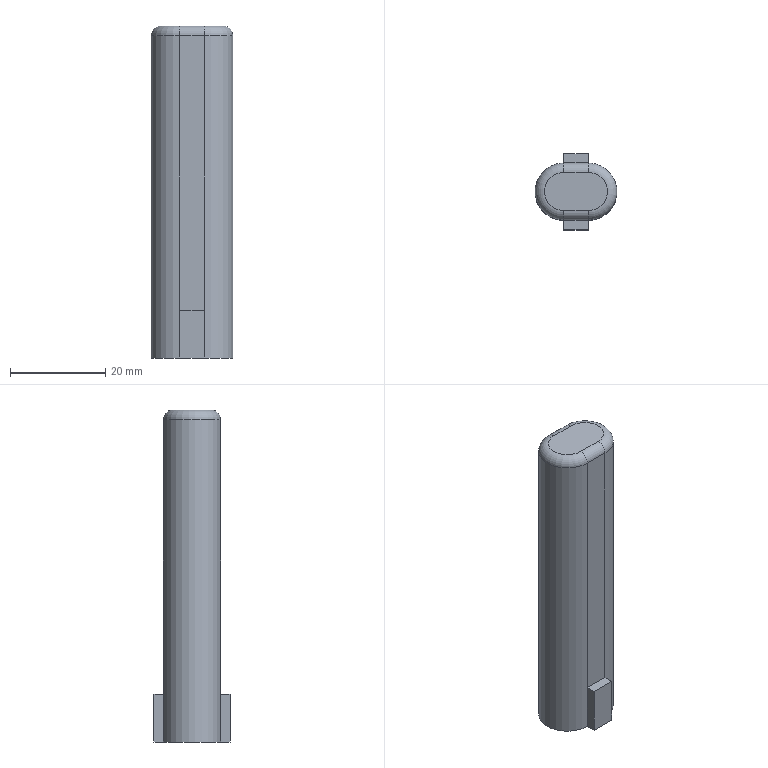Part | STEP file | 1_id1494_x_t | 1 solid | 18 faces | box 17.227 x 16 x 69.85 mm | volume 12451 mm3 | plane 12 | cylinder 4 | torus 2 | commonest cylinder face diameters 4 x2 12 x2
STEP:
#1=CARTESIAN_POINT('',(0.,0.,0.));
#2=DIRECTION('',(0.,0.,1.));
#3=DIRECTION('',(1.,0.,0.));
#4=AXIS2_PLACEMENT_3D('',#1,#2,#3);
#5=CARTESIAN_POINT('',(695.538,183.5,-75.53));
#6=VERTEX_POINT('',#5);
#7=CARTESIAN_POINT('',(695.538,171.5,-75.53));
#8=VERTEX_POINT('',#7);
#9=CARTESIAN_POINT('',(695.538,177.5,-75.53));
#10=DIRECTION('',(0.,0.,-1.));
#11=DIRECTION('',(1.,0.,0.));
#12=AXIS2_PLACEMENT_3D('',#9,#10,#11);
#13=CIRCLE('',#12,6.);
#14=CARTESIAN_POINT('',(695.538,177.5,-5.68));
#15=DIRECTION('',(0.,0.,-1.));
#16=DIRECTION('',(-1.,0.,0.));
#17=AXIS2_PLACEMENT_3D('',#14,#15,#16);
#18=CYLINDRICAL_SURFACE('',#17,6.);
#19=CARTESIAN_POINT('',(-3.142,69.85));
#20=DIRECTION('',(1.,0.));
#21=VECTOR('',#20,1.);
#22=LINE('',#19,#21);
#23=(GEOMETRIC_REPRESENTATION_CONTEXT(2)PARAMETRIC_REPRESENTATION_CONTEXT()REPRESENTATION_CONTEXT('',''));
#24=DEFINITIONAL_REPRESENTATION('',(#22),#23);
#25=PCURVE('',#18,#24);
#26=CARTESIAN_POINT('',(695.538,177.5,-75.53));
#27=DIRECTION('',(0.,0.,1.));
#28=DIRECTION('',(1.,0.,0.));
#29=AXIS2_PLACEMENT_3D('',#26,#27,#28);
#30=PLANE('',#29);
#31=CARTESIAN_POINT('',(6.,-0.000000001));
#32=CARTESIAN_POINT('',(6.,-10.392));
#33=CARTESIAN_POINT('',(-3.,-5.196));
#34=CARTESIAN_POINT('',(-12.,0.000000003));
#35=CARTESIAN_POINT('',(-3.,5.196));
#36=CARTESIAN_POINT('',(6.,10.392));
#37=CARTESIAN_POINT('',(6.,-0.000000001));
#38=(BOUNDED_CURVE()B_SPLINE_CURVE(2,(#31,#32,#33,#34,#35,#36,#37),.UNSPECIFIED.,.T.,.F.)B_SPLINE_CURVE_WITH_KNOTS((1,2,2,2,2,1),(-2.094,0.,2.094,4.189,6.283,8.378),.UNSPECIFIED.)CURVE()GEOMETRIC_REPRESENTATION_ITEM()RATIONAL_B_SPLINE_CURVE((1.,0.5,1.,0.5,1.,0.5,1.))REPRESENTATION_ITEM(''));
#39=(GEOMETRIC_REPRESENTATION_CONTEXT(2)PARAMETRIC_REPRESENTATION_CONTEXT()REPRESENTATION_CONTEXT('',''));
#40=DEFINITIONAL_REPRESENTATION('',(#38),#39);
#41=PCURVE('',#30,#40);
#42=SURFACE_CURVE('',#13,(#25,#41),.PCURVE_S1.);
#43=EDGE_CURVE('',#6,#8,#42,.T.);
#44=ORIENTED_EDGE('',*,*,#43,.F.);
#45=CARTESIAN_POINT('',(695.538,183.5,-65.53));
#46=VERTEX_POINT('',#45);
#47=CARTESIAN_POINT('',(695.538,183.5,-75.53));
#48=DIRECTION('',(0.,0.,1.));
#49=VECTOR('',#48,1.);
#50=LINE('',#47,#49);
#51=CARTESIAN_POINT('',(1.571,69.85));
#52=DIRECTION('',(0.,-1.));
#53=VECTOR('',#52,1.);
#54=LINE('',#51,#53);
#55=(GEOMETRIC_REPRESENTATION_CONTEXT(2)PARAMETRIC_REPRESENTATION_CONTEXT()REPRESENTATION_CONTEXT('',''));
#56=DEFINITIONAL_REPRESENTATION('',(#54),#55);
#57=PCURVE('',#18,#56);
#58=CARTESIAN_POINT('',(695.538,183.5,-75.53));
#59=DIRECTION('',(1.,0.,0.));
#60=DIRECTION('',(0.,0.,-1.));
#61=AXIS2_PLACEMENT_3D('',#58,#59,#60);
#62=PLANE('',#61);
#63=CARTESIAN_POINT('',(0.,0.));
#64=DIRECTION('',(-1.,0.));
#65=VECTOR('',#64,1.);
#66=LINE('',#63,#65);
#67=(GEOMETRIC_REPRESENTATION_CONTEXT(2)PARAMETRIC_REPRESENTATION_CONTEXT()REPRESENTATION_CONTEXT('',''));
#68=DEFINITIONAL_REPRESENTATION('',(#66),#67);
#69=PCURVE('',#62,#68);
#70=SURFACE_CURVE('',#50,(#57,#69),.PCURVE_S1.);
#71=EDGE_CURVE('',#6,#46,#70,.T.);
#72=ORIENTED_EDGE('',*,*,#71,.T.);
#73=CARTESIAN_POINT('',(695.538,183.5,-7.68));
#74=VERTEX_POINT('',#73);
#75=CARTESIAN_POINT('',(695.538,183.5,-65.53));
#76=DIRECTION('',(0.,0.,1.));
#77=VECTOR('',#76,1.);
#78=LINE('',#75,#77);
#79=CARTESIAN_POINT('',(1.571,59.85));
#80=DIRECTION('',(0.,-1.));
#81=VECTOR('',#80,1.);
#82=LINE('',#79,#81);
#83=(GEOMETRIC_REPRESENTATION_CONTEXT(2)PARAMETRIC_REPRESENTATION_CONTEXT()REPRESENTATION_CONTEXT('',''));
#84=DEFINITIONAL_REPRESENTATION('',(#82),#83);
#85=PCURVE('',#18,#84);
#86=CARTESIAN_POINT('',(695.538,183.5,-5.68));
#87=DIRECTION('',(0.,-1.,0.));
#88=DIRECTION('',(0.,0.,1.));
#89=AXIS2_PLACEMENT_3D('',#86,#87,#88);
#90=PLANE('',#89);
#91=CARTESIAN_POINT('',(-59.85,0.));
#92=DIRECTION('',(1.,0.));
#93=VECTOR('',#92,1.);
#94=LINE('',#91,#93);
#95=(GEOMETRIC_REPRESENTATION_CONTEXT(2)PARAMETRIC_REPRESENTATION_CONTEXT()REPRESENTATION_CONTEXT('',''));
#96=DEFINITIONAL_REPRESENTATION('',(#94),#95);
#97=PCURVE('',#90,#96);
#98=SURFACE_CURVE('',#78,(#85,#97),.PCURVE_S1.);
#99=EDGE_CURVE('',#46,#74,#98,.T.);
#100=ORIENTED_EDGE('',*,*,#99,.T.);
#101=CARTESIAN_POINT('',(695.538,171.5,-7.68));
#102=VERTEX_POINT('',#101);
#103=CARTESIAN_POINT('',(695.538,177.5,-7.68));
#104=DIRECTION('',(0.,0.,1.));
#105=DIRECTION('',(0.,-1.,0.));
#106=AXIS2_PLACEMENT_3D('',#103,#104,#105);
#107=CIRCLE('',#106,6.);
#108=CARTESIAN_POINT('',(4.712,2.));
#109=DIRECTION('',(-1.,0.));
#110=VECTOR('',#109,1.);
#111=LINE('',#108,#110);
#112=(GEOMETRIC_REPRESENTATION_CONTEXT(2)PARAMETRIC_REPRESENTATION_CONTEXT()REPRESENTATION_CONTEXT('',''));
#113=DEFINITIONAL_REPRESENTATION('',(#111),#112);
#114=PCURVE('',#18,#113);
#115=CARTESIAN_POINT('',(695.538,177.5,-7.68));
#116=DIRECTION('',(0.,0.,1.));
#117=DIRECTION('',(1.,0.,0.));
#118=AXIS2_PLACEMENT_3D('',#115,#116,#117);
#119=TOROIDAL_SURFACE('',#118,4.,2.);
#120=CARTESIAN_POINT('',(4.712,0.));
#121=DIRECTION('',(1.,0.));
#122=VECTOR('',#121,1.);
#123=LINE('',#120,#122);
#124=(GEOMETRIC_REPRESENTATION_CONTEXT(2)PARAMETRIC_REPRESENTATION_CONTEXT()REPRESENTATION_CONTEXT('',''));
#125=DEFINITIONAL_REPRESENTATION('',(#123),#124);
#126=PCURVE('',#119,#125);
#127=SURFACE_CURVE('',#107,(#114,#126),.PCURVE_S1.);
#128=EDGE_CURVE('',#102,#74,#127,.T.);
#129=ORIENTED_EDGE('',*,*,#128,.F.);
#130=CARTESIAN_POINT('',(695.538,171.5,-65.53));
#131=VERTEX_POINT('',#130);
#132=CARTESIAN_POINT('',(695.538,171.5,-7.68));
#133=DIRECTION('',(0.,0.,-1.));
#134=VECTOR('',#133,1.);
#135=LINE('',#132,#134);
#136=CARTESIAN_POINT('',(4.712,2.));
#137=DIRECTION('',(0.,1.));
#138=VECTOR('',#137,1.);
#139=LINE('',#136,#138);
#140=(GEOMETRIC_REPRESENTATION_CONTEXT(2)PARAMETRIC_REPRESENTATION_CONTEXT()REPRESENTATION_CONTEXT('',''));
#141=DEFINITIONAL_REPRESENTATION('',(#139),#140);
#142=PCURVE('',#18,#141);
#143=CARTESIAN_POINT('',(690.312,171.5,-5.68));
#144=DIRECTION('',(0.,1.,0.));
#145=DIRECTION('',(0.,0.,-1.));
#146=AXIS2_PLACEMENT_3D('',#143,#144,#145);
#147=PLANE('',#146);
#148=CARTESIAN_POINT('',(2.,-5.227));
#149=DIRECTION('',(1.,0.));
#150=VECTOR('',#149,1.);
#151=LINE('',#148,#150);
#152=(GEOMETRIC_REPRESENTATION_CONTEXT(2)PARAMETRIC_REPRESENTATION_CONTEXT()REPRESENTATION_CONTEXT('',''));
#153=DEFINITIONAL_REPRESENTATION('',(#151),#152);
#154=PCURVE('',#147,#153);
#155=SURFACE_CURVE('',#135,(#142,#154),.PCURVE_S1.);
#156=EDGE_CURVE('',#102,#131,#155,.T.);
#157=ORIENTED_EDGE('',*,*,#156,.T.);
#158=CARTESIAN_POINT('',(695.538,171.5,-65.53));
#159=DIRECTION('',(0.,0.,-1.));
#160=VECTOR('',#159,1.);
#161=LINE('',#158,#160);
#162=CARTESIAN_POINT('',(4.712,59.85));
#163=DIRECTION('',(0.,1.));
#164=VECTOR('',#163,1.);
#165=LINE('',#162,#164);
#166=(GEOMETRIC_REPRESENTATION_CONTEXT(2)PARAMETRIC_REPRESENTATION_CONTEXT()REPRESENTATION_CONTEXT('',''));
#167=DEFINITIONAL_REPRESENTATION('',(#165),#166);
#168=PCURVE('',#18,#167);
#169=CARTESIAN_POINT('',(695.538,169.5,-75.53));
#170=DIRECTION('',(1.,0.,0.));
#171=DIRECTION('',(0.,0.,-1.));
#172=AXIS2_PLACEMENT_3D('',#169,#170,#171);
#173=PLANE('',#172);
#174=CARTESIAN_POINT('',(-10.,2.));
#175=DIRECTION('',(1.,0.));
#176=VECTOR('',#175,1.);
#177=LINE('',#174,#176);
#178=(GEOMETRIC_REPRESENTATION_CONTEXT(2)PARAMETRIC_REPRESENTATION_CONTEXT()REPRESENTATION_CONTEXT('',''));
#179=DEFINITIONAL_REPRESENTATION('',(#177),#178);
#180=PCURVE('',#173,#179);
#181=SURFACE_CURVE('',#161,(#168,#180),.PCURVE_S1.);
#182=EDGE_CURVE('',#131,#8,#181,.T.);
#183=ORIENTED_EDGE('',*,*,#182,.T.);
#184=EDGE_LOOP('',(#44,#72,#100,#129,#157,#183));
#185=FACE_BOUND('',#184,.T.);
#186=ADVANCED_FACE('',(#185),#18,.T.);
#187=CARTESIAN_POINT('',(695.538,169.5,-75.53));
#188=VERTEX_POINT('',#187);
#189=CARTESIAN_POINT('',(695.538,171.5,-75.53));
#190=DIRECTION('',(0.,-1.,0.));
#191=VECTOR('',#190,1.);
#192=LINE('',#189,#191);
#193=CARTESIAN_POINT('',(0.,-6.));
#194=DIRECTION('',(0.,-1.));
#195=VECTOR('',#194,1.);
#196=LINE('',#193,#195);
#197=(GEOMETRIC_REPRESENTATION_CONTEXT(2)PARAMETRIC_REPRESENTATION_CONTEXT()REPRESENTATION_CONTEXT('',''));
#198=DEFINITIONAL_REPRESENTATION('',(#196),#197);
#199=PCURVE('',#30,#198);
#200=CARTESIAN_POINT('',(0.,2.));
#201=DIRECTION('',(0.,-1.));
#202=VECTOR('',#201,1.);
#203=LINE('',#200,#202);
#204=(GEOMETRIC_REPRESENTATION_CONTEXT(2)PARAMETRIC_REPRESENTATION_CONTEXT()REPRESENTATION_CONTEXT('',''));
#205=DEFINITIONAL_REPRESENTATION('',(#203),#204);
#206=PCURVE('',#173,#205);
#207=SURFACE_CURVE('',#192,(#199,#206),.PCURVE_S1.);
#208=EDGE_CURVE('',#8,#188,#207,.T.);
#209=ORIENTED_EDGE('',*,*,#208,.T.);
#210=CARTESIAN_POINT('',(690.312,169.5,-75.53));
#211=VERTEX_POINT('',#210);
#212=CARTESIAN_POINT('',(695.538,169.5,-75.53));
#213=DIRECTION('',(-1.,0.,0.));
#214=VECTOR('',#213,1.);
#215=LINE('',#212,#214);
#216=CARTESIAN_POINT('',(0.,-8.));
#217=DIRECTION('',(-1.,0.));
#218=VECTOR('',#217,1.);
#219=LINE('',#216,#218);
#220=(GEOMETRIC_REPRESENTATION_CONTEXT(2)PARAMETRIC_REPRESENTATION_CONTEXT()REPRESENTATION_CONTEXT('',''));
#221=DEFINITIONAL_REPRESENTATION('',(#219),#220);
#222=PCURVE('',#30,#221);
#223=CARTESIAN_POINT('',(690.312,169.5,-75.53));
#224=DIRECTION('',(0.,-1.,0.));
#225=DIRECTION('',(0.,0.,1.));
#226=AXIS2_PLACEMENT_3D('',#223,#224,#225);
#227=PLANE('',#226);
#228=CARTESIAN_POINT('',(0.,-5.227));
#229=DIRECTION('',(0.,1.));
#230=VECTOR('',#229,1.);
#231=LINE('',#228,#230);
#232=(GEOMETRIC_REPRESENTATION_CONTEXT(2)PARAMETRIC_REPRESENTATION_CONTEXT()REPRESENTATION_CONTEXT('',''));
#233=DEFINITIONAL_REPRESENTATION('',(#231),#232);
#234=PCURVE('',#227,#233);
#235=SURFACE_CURVE('',#215,(#222,#234),.PCURVE_S1.);
#236=EDGE_CURVE('',#188,#211,#235,.T.);
#237=ORIENTED_EDGE('',*,*,#236,.T.);
#238=CARTESIAN_POINT('',(690.312,171.5,-75.53));
#239=VERTEX_POINT('',#238);
#240=CARTESIAN_POINT('',(690.312,169.5,-75.53));
#241=DIRECTION('',(0.,1.,0.));
#242=VECTOR('',#241,1.);
#243=LINE('',#240,#242);
#244=CARTESIAN_POINT('',(-5.227,-8.));
#245=DIRECTION('',(0.,1.));
#246=VECTOR('',#245,1.);
#247=LINE('',#244,#246);
#248=(GEOMETRIC_REPRESENTATION_CONTEXT(2)PARAMETRIC_REPRESENTATION_CONTEXT()REPRESENTATION_CONTEXT('',''));
#249=DEFINITIONAL_REPRESENTATION('',(#247),#248);
#250=PCURVE('',#30,#249);
#251=CARTESIAN_POINT('',(690.312,171.5,-75.53));
#252=DIRECTION('',(-1.,0.,0.));
#253=DIRECTION('',(0.,0.,1.));
#254=AXIS2_PLACEMENT_3D('',#251,#252,#253);
#255=PLANE('',#254);
#256=CARTESIAN_POINT('',(0.,-2.));
#257=DIRECTION('',(0.,1.));
#258=VECTOR('',#257,1.);
#259=LINE('',#256,#258);
#260=(GEOMETRIC_REPRESENTATION_CONTEXT(2)PARAMETRIC_REPRESENTATION_CONTEXT()REPRESENTATION_CONTEXT('',''));
#261=DEFINITIONAL_REPRESENTATION('',(#259),#260);
#262=PCURVE('',#255,#261);
#263=SURFACE_CURVE('',#243,(#250,#262),.PCURVE_S1.);
#264=EDGE_CURVE('',#211,#239,#263,.T.);
#265=ORIENTED_EDGE('',*,*,#264,.T.);
#266=CARTESIAN_POINT('',(690.312,183.5,-75.53));
#267=VERTEX_POINT('',#266);
#268=CARTESIAN_POINT('',(690.312,177.5,-75.53));
#269=DIRECTION('',(0.,0.,-1.));
#270=DIRECTION('',(-1.,0.,0.));
#271=AXIS2_PLACEMENT_3D('',#268,#269,#270);
#272=CIRCLE('',#271,6.);
#273=CARTESIAN_POINT('',(-11.227,0.));
#274=CARTESIAN_POINT('',(-11.227,10.392));
#275=CARTESIAN_POINT('',(-2.227,5.196));
#276=CARTESIAN_POINT('',(6.773,0.));
#277=CARTESIAN_POINT('',(-2.227,-5.196));
#278=CARTESIAN_POINT('',(-11.227,-10.392));
#279=CARTESIAN_POINT('',(-11.227,0.));
#280=(BOUNDED_CURVE()B_SPLINE_CURVE(2,(#273,#274,#275,#276,#277,#278,#279),.UNSPECIFIED.,.T.,.F.)B_SPLINE_CURVE_WITH_KNOTS((1,2,2,2,2,1),(-2.094,0.,2.094,4.189,6.283,8.378),.UNSPECIFIED.)CURVE()GEOMETRIC_REPRESENTATION_ITEM()RATIONAL_B_SPLINE_CURVE((1.,0.5,1.,0.5,1.,0.5,1.))REPRESENTATION_ITEM(''));
#281=(GEOMETRIC_REPRESENTATION_CONTEXT(2)PARAMETRIC_REPRESENTATION_CONTEXT()REPRESENTATION_CONTEXT('',''));
#282=DEFINITIONAL_REPRESENTATION('',(#280),#281);
#283=PCURVE('',#30,#282);
#284=CARTESIAN_POINT('',(690.312,177.5,-5.68));
#285=DIRECTION('',(0.,0.,-1.));
#286=DIRECTION('',(-1.,0.,0.));
#287=AXIS2_PLACEMENT_3D('',#284,#285,#286);
#288=CYLINDRICAL_SURFACE('',#287,6.);
#289=CARTESIAN_POINT('',(-6.283,69.85));
#290=DIRECTION('',(1.,0.));
#291=VECTOR('',#290,1.);
#292=LINE('',#289,#291);
#293=(GEOMETRIC_REPRESENTATION_CONTEXT(2)PARAMETRIC_REPRESENTATION_CONTEXT()REPRESENTATION_CONTEXT('',''));
#294=DEFINITIONAL_REPRESENTATION('',(#292),#293);
#295=PCURVE('',#288,#294);
#296=SURFACE_CURVE('',#272,(#283,#295),.PCURVE_S1.);
#297=EDGE_CURVE('',#239,#267,#296,.T.);
#298=ORIENTED_EDGE('',*,*,#297,.T.);
#299=CARTESIAN_POINT('',(690.312,185.5,-75.53));
#300=VERTEX_POINT('',#299);
#301=CARTESIAN_POINT('',(690.312,183.5,-75.53));
#302=DIRECTION('',(0.,1.,0.));
#303=VECTOR('',#302,1.);
#304=LINE('',#301,#303);
#305=CARTESIAN_POINT('',(-5.227,6.));
#306=DIRECTION('',(0.,1.));
#307=VECTOR('',#306,1.);
#308=LINE('',#305,#307);
#309=(GEOMETRIC_REPRESENTATION_CONTEXT(2)PARAMETRIC_REPRESENTATION_CONTEXT()REPRESENTATION_CONTEXT('',''));
#310=DEFINITIONAL_REPRESENTATION('',(#308),#309);
#311=PCURVE('',#30,#310);
#312=CARTESIAN_POINT('',(690.312,185.5,-75.53));
#313=DIRECTION('',(-1.,0.,0.));
#314=DIRECTION('',(0.,0.,1.));
#315=AXIS2_PLACEMENT_3D('',#312,#313,#314);
#316=PLANE('',#315);
#317=CARTESIAN_POINT('',(0.,-2.));
#318=DIRECTION('',(0.,1.));
#319=VECTOR('',#318,1.);
#320=LINE('',#317,#319);
#321=(GEOMETRIC_REPRESENTATION_CONTEXT(2)PARAMETRIC_REPRESENTATION_CONTEXT()REPRESENTATION_CONTEXT('',''));
#322=DEFINITIONAL_REPRESENTATION('',(#320),#321);
#323=PCURVE('',#316,#322);
#324=SURFACE_CURVE('',#304,(#311,#323),.PCURVE_S1.);
#325=EDGE_CURVE('',#267,#300,#324,.T.);
#326=ORIENTED_EDGE('',*,*,#325,.T.);
#327=CARTESIAN_POINT('',(695.538,185.5,-75.53));
#328=VERTEX_POINT('',#327);
#329=CARTESIAN_POINT('',(690.312,185.5,-75.53));
#330=DIRECTION('',(1.,0.,0.));
#331=VECTOR('',#330,1.);
#332=LINE('',#329,#331);
#333=CARTESIAN_POINT('',(-5.227,8.));
#334=DIRECTION('',(1.,0.));
#335=VECTOR('',#334,1.);
#336=LINE('',#333,#335);
#337=(GEOMETRIC_REPRESENTATION_CONTEXT(2)PARAMETRIC_REPRESENTATION_CONTEXT()REPRESENTATION_CONTEXT('',''));
#338=DEFINITIONAL_REPRESENTATION('',(#336),#337);
#339=PCURVE('',#30,#338);
#340=CARTESIAN_POINT('',(695.538,185.5,-75.53));
#341=DIRECTION('',(0.,1.,0.));
#342=DIRECTION('',(0.,0.,-1.));
#343=AXIS2_PLACEMENT_3D('',#340,#341,#342);
#344=PLANE('',#343);
#345=CARTESIAN_POINT('',(0.,5.227));
#346=DIRECTION('',(0.,-1.));
#347=VECTOR('',#346,1.);
#348=LINE('',#345,#347);
#349=(GEOMETRIC_REPRESENTATION_CONTEXT(2)PARAMETRIC_REPRESENTATION_CONTEXT()REPRESENTATION_CONTEXT('',''));
#350=DEFINITIONAL_REPRESENTATION('',(#348),#349);
#351=PCURVE('',#344,#350);
#352=SURFACE_CURVE('',#332,(#339,#351),.PCURVE_S1.);
#353=EDGE_CURVE('',#300,#328,#352,.T.);
#354=ORIENTED_EDGE('',*,*,#353,.T.);
#355=CARTESIAN_POINT('',(695.538,185.5,-75.53));
#356=DIRECTION('',(0.,-1.,0.));
#357=VECTOR('',#356,1.);
#358=LINE('',#355,#357);
#359=CARTESIAN_POINT('',(0.,8.));
#360=DIRECTION('',(0.,-1.));
#361=VECTOR('',#360,1.);
#362=LINE('',#359,#361);
#363=(GEOMETRIC_REPRESENTATION_CONTEXT(2)PARAMETRIC_REPRESENTATION_CONTEXT()REPRESENTATION_CONTEXT('',''));
#364=DEFINITIONAL_REPRESENTATION('',(#362),#363);
#365=PCURVE('',#30,#364);
#366=CARTESIAN_POINT('',(0.,2.));
#367=DIRECTION('',(0.,-1.));
#368=VECTOR('',#367,1.);
#369=LINE('',#366,#368);
#370=(GEOMETRIC_REPRESENTATION_CONTEXT(2)PARAMETRIC_REPRESENTATION_CONTEXT()REPRESENTATION_CONTEXT('',''));
#371=DEFINITIONAL_REPRESENTATION('',(#369),#370);
#372=PCURVE('',#62,#371);
#373=SURFACE_CURVE('',#358,(#365,#372),.PCURVE_S1.);
#374=EDGE_CURVE('',#328,#6,#373,.T.);
#375=ORIENTED_EDGE('',*,*,#374,.T.);
#376=ORIENTED_EDGE('',*,*,#43,.T.);
#377=EDGE_LOOP('',(#209,#237,#265,#298,#326,#354,#375,#376));
#378=FACE_BOUND('',#377,.T.);
#379=ADVANCED_FACE('',(#378),#30,.F.);
#380=ORIENTED_EDGE('',*,*,#71,.F.);
#381=ORIENTED_EDGE('',*,*,#374,.F.);
#382=CARTESIAN_POINT('',(695.538,185.5,-65.53));
#383=VERTEX_POINT('',#382);
#384=CARTESIAN_POINT('',(695.538,185.5,-65.53));
#385=DIRECTION('',(0.,0.,-1.));
#386=VECTOR('',#385,1.);
#387=LINE('',#384,#386);
#388=CARTESIAN_POINT('',(-10.,2.));
#389=DIRECTION('',(1.,0.));
#390=VECTOR('',#389,1.);
#391=LINE('',#388,#390);
#392=(GEOMETRIC_REPRESENTATION_CONTEXT(2)PARAMETRIC_REPRESENTATION_CONTEXT()REPRESENTATION_CONTEXT('',''));
#393=DEFINITIONAL_REPRESENTATION('',(#391),#392);
#394=PCURVE('',#62,#393);
#395=CARTESIAN_POINT('',(-10.,0.));
#396=DIRECTION('',(1.,0.));
#397=VECTOR('',#396,1.);
#398=LINE('',#395,#397);
#399=(GEOMETRIC_REPRESENTATION_CONTEXT(2)PARAMETRIC_REPRESENTATION_CONTEXT()REPRESENTATION_CONTEXT('',''));
#400=DEFINITIONAL_REPRESENTATION('',(#398),#399);
#401=PCURVE('',#344,#400);
#402=SURFACE_CURVE('',#387,(#394,#401),.PCURVE_S1.);
#403=EDGE_CURVE('',#383,#328,#402,.T.);
#404=ORIENTED_EDGE('',*,*,#403,.F.);
#405=CARTESIAN_POINT('',(695.538,185.5,-65.53));
#406=DIRECTION('',(0.,-1.,0.));
#407=VECTOR('',#406,1.);
#408=LINE('',#405,#407);
#409=CARTESIAN_POINT('',(-10.,2.));
#410=DIRECTION('',(0.,-1.));
#411=VECTOR('',#410,1.);
#412=LINE('',#409,#411);
#413=(GEOMETRIC_REPRESENTATION_CONTEXT(2)PARAMETRIC_REPRESENTATION_CONTEXT()REPRESENTATION_CONTEXT('',''));
#414=DEFINITIONAL_REPRESENTATION('',(#412),#413);
#415=PCURVE('',#62,#414);
#416=CARTESIAN_POINT('',(690.312,185.5,-65.53));
#417=DIRECTION('',(0.,0.,1.));
#418=DIRECTION('',(1.,0.,0.));
#419=AXIS2_PLACEMENT_3D('',#416,#417,#418);
#420=PLANE('',#419);
#421=CARTESIAN_POINT('',(5.227,0.));
#422=DIRECTION('',(0.,-1.));
#423=VECTOR('',#422,1.);
#424=LINE('',#421,#423);
#425=(GEOMETRIC_REPRESENTATION_CONTEXT(2)PARAMETRIC_REPRESENTATION_CONTEXT()REPRESENTATION_CONTEXT('',''));
#426=DEFINITIONAL_REPRESENTATION('',(#424),#425);
#427=PCURVE('',#420,#426);
#428=SURFACE_CURVE('',#408,(#415,#427),.PCURVE_S1.);
#429=EDGE_CURVE('',#383,#46,#428,.T.);
#430=ORIENTED_EDGE('',*,*,#429,.T.);
#431=EDGE_LOOP('',(#380,#381,#404,#430));
#432=FACE_BOUND('',#431,.T.);
#433=ADVANCED_FACE('',(#432),#62,.T.);
#434=CARTESIAN_POINT('',(690.312,183.5,-65.53));
#435=VERTEX_POINT('',#434);
#436=CARTESIAN_POINT('',(690.312,185.5,-65.53));
#437=VERTEX_POINT('',#436);
#438=CARTESIAN_POINT('',(690.312,183.5,-65.53));
#439=DIRECTION('',(0.,1.,0.));
#440=VECTOR('',#439,1.);
#441=LINE('',#438,#440);
#442=CARTESIAN_POINT('',(0.,-2.));
#443=DIRECTION('',(0.,1.));
#444=VECTOR('',#443,1.);
#445=LINE('',#442,#444);
#446=(GEOMETRIC_REPRESENTATION_CONTEXT(2)PARAMETRIC_REPRESENTATION_CONTEXT()REPRESENTATION_CONTEXT('',''));
#447=DEFINITIONAL_REPRESENTATION('',(#445),#446);
#448=PCURVE('',#420,#447);
#449=CARTESIAN_POINT('',(10.,-2.));
#450=DIRECTION('',(0.,1.));
#451=VECTOR('',#450,1.);
#452=LINE('',#449,#451);
#453=(GEOMETRIC_REPRESENTATION_CONTEXT(2)PARAMETRIC_REPRESENTATION_CONTEXT()REPRESENTATION_CONTEXT('',''));
#454=DEFINITIONAL_REPRESENTATION('',(#452),#453);
#455=PCURVE('',#316,#454);
#456=SURFACE_CURVE('',#441,(#448,#455),.PCURVE_S1.);
#457=EDGE_CURVE('',#435,#437,#456,.T.);
#458=ORIENTED_EDGE('',*,*,#457,.F.);
#459=CARTESIAN_POINT('',(695.538,183.5,-65.53));
#460=DIRECTION('',(-1.,0.,0.));
#461=VECTOR('',#460,1.);
#462=LINE('',#459,#461);
#463=CARTESIAN_POINT('',(5.227,-2.));
#464=DIRECTION('',(-1.,0.));
#465=VECTOR('',#464,1.);
#466=LINE('',#463,#465);
#467=(GEOMETRIC_REPRESENTATION_CONTEXT(2)PARAMETRIC_REPRESENTATION_CONTEXT()REPRESENTATION_CONTEXT('',''));
#468=DEFINITIONAL_REPRESENTATION('',(#466),#467);
#469=PCURVE('',#420,#468);
#470=CARTESIAN_POINT('',(-59.85,0.));
#471=DIRECTION('',(0.,1.));
#472=VECTOR('',#471,1.);
#473=LINE('',#470,#472);
#474=(GEOMETRIC_REPRESENTATION_CONTEXT(2)PARAMETRIC_REPRESENTATION_CONTEXT()REPRESENTATION_CONTEXT('',''));
#475=DEFINITIONAL_REPRESENTATION('',(#473),#474);
#476=PCURVE('',#90,#475);
#477=SURFACE_CURVE('',#462,(#469,#476),.PCURVE_S1.);
#478=EDGE_CURVE('',#46,#435,#477,.T.);
#479=ORIENTED_EDGE('',*,*,#478,.F.);
#480=ORIENTED_EDGE('',*,*,#429,.F.);
#481=CARTESIAN_POINT('',(690.312,185.5,-65.53));
#482=DIRECTION('',(1.,0.,0.));
#483=VECTOR('',#482,1.);
#484=LINE('',#481,#483);
#485=CARTESIAN_POINT('',(0.,0.));
#486=DIRECTION('',(1.,0.));
#487=VECTOR('',#486,1.);
#488=LINE('',#485,#487);
#489=(GEOMETRIC_REPRESENTATION_CONTEXT(2)PARAMETRIC_REPRESENTATION_CONTEXT()REPRESENTATION_CONTEXT('',''));
#490=DEFINITIONAL_REPRESENTATION('',(#488),#489);
#491=PCURVE('',#420,#490);
#492=CARTESIAN_POINT('',(-10.,5.227));
#493=DIRECTION('',(0.,-1.));
#494=VECTOR('',#493,1.);
#495=LINE('',#492,#494);
#496=(GEOMETRIC_REPRESENTATION_CONTEXT(2)PARAMETRIC_REPRESENTATION_CONTEXT()REPRESENTATION_CONTEXT('',''));
#497=DEFINITIONAL_REPRESENTATION('',(#495),#496);
#498=PCURVE('',#344,#497);
#499=SURFACE_CURVE('',#484,(#491,#498),.PCURVE_S1.);
#500=EDGE_CURVE('',#437,#383,#499,.T.);
#501=ORIENTED_EDGE('',*,*,#500,.F.);
#502=EDGE_LOOP('',(#458,#479,#480,#501));
#503=FACE_BOUND('',#502,.T.);
#504=ADVANCED_FACE('',(#503),#420,.T.);
#505=ORIENTED_EDGE('',*,*,#403,.T.);
#506=ORIENTED_EDGE('',*,*,#353,.F.);
#507=CARTESIAN_POINT('',(690.312,185.5,-65.53));
#508=DIRECTION('',(0.,0.,-1.));
#509=VECTOR('',#508,1.);
#510=LINE('',#507,#509);
#511=CARTESIAN_POINT('',(-10.,5.227));
#512=DIRECTION('',(1.,0.));
#513=VECTOR('',#512,1.);
#514=LINE('',#511,#513);
#515=(GEOMETRIC_REPRESENTATION_CONTEXT(2)PARAMETRIC_REPRESENTATION_CONTEXT()REPRESENTATION_CONTEXT('',''));
#516=DEFINITIONAL_REPRESENTATION('',(#514),#515);
#517=PCURVE('',#344,#516);
#518=CARTESIAN_POINT('',(10.,0.));
#519=DIRECTION('',(-1.,0.));
#520=VECTOR('',#519,1.);
#521=LINE('',#518,#520);
#522=(GEOMETRIC_REPRESENTATION_CONTEXT(2)PARAMETRIC_REPRESENTATION_CONTEXT()REPRESENTATION_CONTEXT('',''));
#523=DEFINITIONAL_REPRESENTATION('',(#521),#522);
#524=PCURVE('',#316,#523);
#525=SURFACE_CURVE('',#510,(#517,#524),.PCURVE_S1.);
#526=EDGE_CURVE('',#437,#300,#525,.T.);
#527=ORIENTED_EDGE('',*,*,#526,.F.);
#528=ORIENTED_EDGE('',*,*,#500,.T.);
#529=EDGE_LOOP('',(#505,#506,#527,#528));
#530=FACE_BOUND('',#529,.T.);
#531=ADVANCED_FACE('',(#530),#344,.T.);
#532=ORIENTED_EDGE('',*,*,#526,.T.);
#533=ORIENTED_EDGE('',*,*,#325,.F.);
#534=CARTESIAN_POINT('',(690.312,183.5,-65.53));
#535=DIRECTION('',(0.,0.,-1.));
#536=VECTOR('',#535,1.);
#537=LINE('',#534,#536);
#538=CARTESIAN_POINT('',(10.,-2.));
#539=DIRECTION('',(-1.,0.));
#540=VECTOR('',#539,1.);
#541=LINE('',#538,#540);
#542=(GEOMETRIC_REPRESENTATION_CONTEXT(2)PARAMETRIC_REPRESENTATION_CONTEXT()REPRESENTATION_CONTEXT('',''));
#543=DEFINITIONAL_REPRESENTATION('',(#541),#542);
#544=PCURVE('',#316,#543);
#545=CARTESIAN_POINT('',(1.571,59.85));
#546=DIRECTION('',(0.,1.));
#547=VECTOR('',#546,1.);
#548=LINE('',#545,#547);
#549=(GEOMETRIC_REPRESENTATION_CONTEXT(2)PARAMETRIC_REPRESENTATION_CONTEXT()REPRESENTATION_CONTEXT('',''));
#550=DEFINITIONAL_REPRESENTATION('',(#548),#549);
#551=PCURVE('',#288,#550);
#552=SURFACE_CURVE('',#537,(#544,#551),.PCURVE_S1.);
#553=EDGE_CURVE('',#435,#267,#552,.T.);
#554=ORIENTED_EDGE('',*,*,#553,.F.);
#555=ORIENTED_EDGE('',*,*,#457,.T.);
#556=EDGE_LOOP('',(#532,#533,#554,#555));
#557=FACE_BOUND('',#556,.T.);
#558=ADVANCED_FACE('',(#557),#316,.T.);
#559=CARTESIAN_POINT('',(690.312,183.5,-7.68));
#560=VERTEX_POINT('',#559);
#561=CARTESIAN_POINT('',(690.312,171.5,-7.68));
#562=VERTEX_POINT('',#561);
#563=CARTESIAN_POINT('',(690.312,177.5,-7.68));
#564=DIRECTION('',(0.,0.,1.));
#565=DIRECTION('',(-1.,0.,0.));
#566=AXIS2_PLACEMENT_3D('',#563,#564,#565);
#567=CIRCLE('',#566,6.);
#568=CARTESIAN_POINT('',(6.283,2.));
#569=DIRECTION('',(-1.,0.));
#570=VECTOR('',#569,1.);
#571=LINE('',#568,#570);
#572=(GEOMETRIC_REPRESENTATION_CONTEXT(2)PARAMETRIC_REPRESENTATION_CONTEXT()REPRESENTATION_CONTEXT('',''));
#573=DEFINITIONAL_REPRESENTATION('',(#571),#572);
#574=PCURVE('',#288,#573);
#575=CARTESIAN_POINT('',(690.312,177.5,-7.68));
#576=DIRECTION('',(0.,0.,1.));
#577=DIRECTION('',(1.,0.,0.));
#578=AXIS2_PLACEMENT_3D('',#575,#576,#577);
#579=TOROIDAL_SURFACE('',#578,4.,2.);
#580=CARTESIAN_POINT('',(-3.142,0.));
#581=DIRECTION('',(1.,0.));
#582=VECTOR('',#581,1.);
#583=LINE('',#580,#582);
#584=(GEOMETRIC_REPRESENTATION_CONTEXT(2)PARAMETRIC_REPRESENTATION_CONTEXT()REPRESENTATION_CONTEXT('',''));
#585=DEFINITIONAL_REPRESENTATION('',(#583),#584);
#586=PCURVE('',#579,#585);
#587=SURFACE_CURVE('',#567,(#574,#586),.PCURVE_S1.);
#588=EDGE_CURVE('',#560,#562,#587,.T.);
#589=ORIENTED_EDGE('',*,*,#588,.F.);
#590=CARTESIAN_POINT('',(690.312,183.5,-7.68));
#591=DIRECTION('',(0.,0.,-1.));
#592=VECTOR('',#591,1.);
#593=LINE('',#590,#592);
#594=CARTESIAN_POINT('',(1.571,2.));
#595=DIRECTION('',(0.,1.));
#596=VECTOR('',#595,1.);
#597=LINE('',#594,#596);
#598=(GEOMETRIC_REPRESENTATION_CONTEXT(2)PARAMETRIC_REPRESENTATION_CONTEXT()REPRESENTATION_CONTEXT('',''));
#599=DEFINITIONAL_REPRESENTATION('',(#597),#598);
#600=PCURVE('',#288,#599);
#601=CARTESIAN_POINT('',(-2.,5.227));
#602=DIRECTION('',(-1.,0.));
#603=VECTOR('',#602,1.);
#604=LINE('',#601,#603);
#605=(GEOMETRIC_REPRESENTATION_CONTEXT(2)PARAMETRIC_REPRESENTATION_CONTEXT()REPRESENTATION_CONTEXT('',''));
#606=DEFINITIONAL_REPRESENTATION('',(#604),#605);
#607=PCURVE('',#90,#606);
#608=SURFACE_CURVE('',#593,(#600,#607),.PCURVE_S1.);
#609=EDGE_CURVE('',#560,#435,#608,.T.);
#610=ORIENTED_EDGE('',*,*,#609,.T.);
#611=ORIENTED_EDGE('',*,*,#553,.T.);
#612=ORIENTED_EDGE('',*,*,#297,.F.);
#613=CARTESIAN_POINT('',(690.312,171.5,-65.53));
#614=VERTEX_POINT('',#613);
#615=CARTESIAN_POINT('',(690.312,171.5,-75.53));
#616=DIRECTION('',(0.,0.,1.));
#617=VECTOR('',#616,1.);
#618=LINE('',#615,#617);
#619=CARTESIAN_POINT('',(-1.571,69.85));
#620=DIRECTION('',(0.,-1.));
#621=VECTOR('',#620,1.);
#622=LINE('',#619,#621);
#623=(GEOMETRIC_REPRESENTATION_CONTEXT(2)PARAMETRIC_REPRESENTATION_CONTEXT()REPRESENTATION_CONTEXT('',''));
#624=DEFINITIONAL_REPRESENTATION('',(#622),#623);
#625=PCURVE('',#288,#624);
#626=CARTESIAN_POINT('',(0.,0.));
#627=DIRECTION('',(1.,0.));
#628=VECTOR('',#627,1.);
#629=LINE('',#626,#628);
#630=(GEOMETRIC_REPRESENTATION_CONTEXT(2)PARAMETRIC_REPRESENTATION_CONTEXT()REPRESENTATION_CONTEXT('',''));
#631=DEFINITIONAL_REPRESENTATION('',(#629),#630);
#632=PCURVE('',#255,#631);
#633=SURFACE_CURVE('',#618,(#625,#632),.PCURVE_S1.);
#634=EDGE_CURVE('',#239,#614,#633,.T.);
#635=ORIENTED_EDGE('',*,*,#634,.T.);
#636=CARTESIAN_POINT('',(690.312,171.5,-65.53));
#637=DIRECTION('',(0.,0.,1.));
#638=VECTOR('',#637,1.);
#639=LINE('',#636,#638);
#640=CARTESIAN_POINT('',(-1.571,59.85));
#641=DIRECTION('',(0.,-1.));
#642=VECTOR('',#641,1.);
#643=LINE('',#640,#642);
#644=(GEOMETRIC_REPRESENTATION_CONTEXT(2)PARAMETRIC_REPRESENTATION_CONTEXT()REPRESENTATION_CONTEXT('',''));
#645=DEFINITIONAL_REPRESENTATION('',(#643),#644);
#646=PCURVE('',#288,#645);
#647=CARTESIAN_POINT('',(59.85,0.));
#648=DIRECTION('',(-1.,0.));
#649=VECTOR('',#648,1.);
#650=LINE('',#647,#649);
#651=(GEOMETRIC_REPRESENTATION_CONTEXT(2)PARAMETRIC_REPRESENTATION_CONTEXT()REPRESENTATION_CONTEXT('',''));
#652=DEFINITIONAL_REPRESENTATION('',(#650),#651);
#653=PCURVE('',#147,#652);
#654=SURFACE_CURVE('',#639,(#646,#653),.PCURVE_S1.);
#655=EDGE_CURVE('',#614,#562,#654,.T.);
#656=ORIENTED_EDGE('',*,*,#655,.T.);
#657=EDGE_LOOP('',(#589,#610,#611,#612,#635,#656));
#658=FACE_BOUND('',#657,.T.);
#659=ADVANCED_FACE('',(#658),#288,.T.);
#660=CARTESIAN_POINT('',(690.312,181.5,-5.68));
#661=VERTEX_POINT('',#660);
#662=CARTESIAN_POINT('',(690.312,181.5,-7.68));
#663=DIRECTION('',(-1.,0.,0.));
#664=DIRECTION('',(0.,0.,1.));
#665=AXIS2_PLACEMENT_3D('',#662,#663,#664);
#666=CIRCLE('',#665,2.);
#667=CARTESIAN_POINT('',(1.571,1.571));
#668=DIRECTION('',(0.,-1.));
#669=VECTOR('',#668,1.);
#670=LINE('',#667,#669);
#671=(GEOMETRIC_REPRESENTATION_CONTEXT(2)PARAMETRIC_REPRESENTATION_CONTEXT()REPRESENTATION_CONTEXT('',''));
#672=DEFINITIONAL_REPRESENTATION('',(#670),#671);
#673=PCURVE('',#579,#672);
#674=CARTESIAN_POINT('',(695.538,181.5,-7.68));
#675=DIRECTION('',(1.,0.,0.));
#676=DIRECTION('',(0.,0.,-1.));
#677=AXIS2_PLACEMENT_3D('',#674,#675,#676);
#678=CYLINDRICAL_SURFACE('',#677,2.);
#679=CARTESIAN_POINT('',(3.142,-5.227));
#680=DIRECTION('',(-1.,0.));
#681=VECTOR('',#680,1.);
#682=LINE('',#679,#681);
#683=(GEOMETRIC_REPRESENTATION_CONTEXT(2)PARAMETRIC_REPRESENTATION_CONTEXT()REPRESENTATION_CONTEXT('',''));
#684=DEFINITIONAL_REPRESENTATION('',(#682),#683);
#685=PCURVE('',#678,#684);
#686=SURFACE_CURVE('',#666,(#673,#685),.PCURVE_S1.);
#687=EDGE_CURVE('',#661,#560,#686,.T.);
#688=ORIENTED_EDGE('',*,*,#687,.T.);
#689=ORIENTED_EDGE('',*,*,#588,.T.);
#690=CARTESIAN_POINT('',(690.312,173.5,-5.68));
#691=VERTEX_POINT('',#690);
#692=CARTESIAN_POINT('',(690.312,173.5,-7.68));
#693=DIRECTION('',(-1.,0.,0.));
#694=DIRECTION('',(0.,-1.,0.));
#695=AXIS2_PLACEMENT_3D('',#692,#693,#694);
#696=CIRCLE('',#695,2.);
#697=CARTESIAN_POINT('',(4.712,0.));
#698=DIRECTION('',(0.,1.));
#699=VECTOR('',#698,1.);
#700=LINE('',#697,#699);
#701=(GEOMETRIC_REPRESENTATION_CONTEXT(2)PARAMETRIC_REPRESENTATION_CONTEXT()REPRESENTATION_CONTEXT('',''));
#702=DEFINITIONAL_REPRESENTATION('',(#700),#701);
#703=PCURVE('',#579,#702);
#704=CARTESIAN_POINT('',(695.538,173.5,-7.68));
#705=DIRECTION('',(-1.,0.,0.));
#706=DIRECTION('',(0.,0.,1.));
#707=AXIS2_PLACEMENT_3D('',#704,#705,#706);
#708=CYLINDRICAL_SURFACE('',#707,2.);
#709=CARTESIAN_POINT('',(4.712,5.227));
#710=DIRECTION('',(1.,0.));
#711=VECTOR('',#710,1.);
#712=LINE('',#709,#711);
#713=(GEOMETRIC_REPRESENTATION_CONTEXT(2)PARAMETRIC_REPRESENTATION_CONTEXT()REPRESENTATION_CONTEXT('',''));
#714=DEFINITIONAL_REPRESENTATION('',(#712),#713);
#715=PCURVE('',#708,#714);
#716=SURFACE_CURVE('',#696,(#703,#715),.PCURVE_S1.);
#717=EDGE_CURVE('',#562,#691,#716,.T.);
#718=ORIENTED_EDGE('',*,*,#717,.T.);
#719=CARTESIAN_POINT('',(690.312,177.5,-5.68));
#720=DIRECTION('',(0.,0.,1.));
#721=DIRECTION('',(0.,1.,0.));
#722=AXIS2_PLACEMENT_3D('',#719,#720,#721);
#723=CIRCLE('',#722,4.);
#724=CARTESIAN_POINT('',(1.571,1.571));
#725=DIRECTION('',(1.,0.));
#726=VECTOR('',#725,1.);
#727=LINE('',#724,#726);
#728=(GEOMETRIC_REPRESENTATION_CONTEXT(2)PARAMETRIC_REPRESENTATION_CONTEXT()REPRESENTATION_CONTEXT('',''));
#729=DEFINITIONAL_REPRESENTATION('',(#727),#728);
#730=PCURVE('',#579,#729);
#731=CARTESIAN_POINT('',(695.538,177.5,-5.68));
#732=DIRECTION('',(0.,0.,1.));
#733=DIRECTION('',(1.,0.,0.));
#734=AXIS2_PLACEMENT_3D('',#731,#732,#733);
#735=PLANE('',#734);
#736=CARTESIAN_POINT('',(-5.227,0.));
#737=DIRECTION('',(0.,1.));
#738=AXIS2_PLACEMENT_2D('',#736,#737);
#739=CIRCLE('',#738,4.);
#740=(GEOMETRIC_REPRESENTATION_CONTEXT(2)PARAMETRIC_REPRESENTATION_CONTEXT()REPRESENTATION_CONTEXT('',''));
#741=DEFINITIONAL_REPRESENTATION('',(#739),#740);
#742=PCURVE('',#735,#741);
#743=SURFACE_CURVE('',#723,(#730,#742),.PCURVE_S1.);
#744=EDGE_CURVE('',#661,#691,#743,.T.);
#745=ORIENTED_EDGE('',*,*,#744,.F.);
#746=EDGE_LOOP('',(#688,#689,#718,#745));
#747=FACE_BOUND('',#746,.T.);
#748=ADVANCED_FACE('',(#747),#579,.T.);
#749=CARTESIAN_POINT('',(695.538,173.5,-5.68));
#750=VERTEX_POINT('',#749);
#751=CARTESIAN_POINT('',(695.538,181.5,-5.68));
#752=VERTEX_POINT('',#751);
#753=CARTESIAN_POINT('',(695.538,177.5,-5.68));
#754=DIRECTION('',(0.,0.,1.));
#755=DIRECTION('',(0.,-1.,0.));
#756=AXIS2_PLACEMENT_3D('',#753,#754,#755);
#757=CIRCLE('',#756,4.);
#758=CARTESIAN_POINT('',(0.,0.));
#759=DIRECTION('',(0.,-1.));
#760=AXIS2_PLACEMENT_2D('',#758,#759);
#761=CIRCLE('',#760,4.);
#762=(GEOMETRIC_REPRESENTATION_CONTEXT(2)PARAMETRIC_REPRESENTATION_CONTEXT()REPRESENTATION_CONTEXT('',''));
#763=DEFINITIONAL_REPRESENTATION('',(#761),#762);
#764=PCURVE('',#735,#763);
#765=CARTESIAN_POINT('',(4.712,1.571));
#766=DIRECTION('',(1.,0.));
#767=VECTOR('',#766,1.);
#768=LINE('',#765,#767);
#769=(GEOMETRIC_REPRESENTATION_CONTEXT(2)PARAMETRIC_REPRESENTATION_CONTEXT()REPRESENTATION_CONTEXT('',''));
#770=DEFINITIONAL_REPRESENTATION('',(#768),#769);
#771=PCURVE('',#119,#770);
#772=SURFACE_CURVE('',#757,(#764,#771),.PCURVE_S1.);
#773=EDGE_CURVE('',#750,#752,#772,.T.);
#774=ORIENTED_EDGE('',*,*,#773,.T.);
#775=CARTESIAN_POINT('',(690.312,181.5,-5.68));
#776=DIRECTION('',(1.,0.,0.));
#777=VECTOR('',#776,1.);
#778=LINE('',#775,#777);
#779=CARTESIAN_POINT('',(-5.227,4.));
#780=DIRECTION('',(1.,0.));
#781=VECTOR('',#780,1.);
#782=LINE('',#779,#781);
#783=(GEOMETRIC_REPRESENTATION_CONTEXT(2)PARAMETRIC_REPRESENTATION_CONTEXT()REPRESENTATION_CONTEXT('',''));
#784=DEFINITIONAL_REPRESENTATION('',(#782),#783);
#785=PCURVE('',#735,#784);
#786=CARTESIAN_POINT('',(3.142,-5.227));
#787=DIRECTION('',(0.,1.));
#788=VECTOR('',#787,1.);
#789=LINE('',#786,#788);
#790=(GEOMETRIC_REPRESENTATION_CONTEXT(2)PARAMETRIC_REPRESENTATION_CONTEXT()REPRESENTATION_CONTEXT('',''));
#791=DEFINITIONAL_REPRESENTATION('',(#789),#790);
#792=PCURVE('',#678,#791);
#793=SURFACE_CURVE('',#778,(#785,#792),.PCURVE_S1.);
#794=EDGE_CURVE('',#661,#752,#793,.T.);
#795=ORIENTED_EDGE('',*,*,#794,.F.);
#796=ORIENTED_EDGE('',*,*,#744,.T.);
#797=CARTESIAN_POINT('',(695.538,173.5,-5.68));
#798=DIRECTION('',(-1.,0.,0.));
#799=VECTOR('',#798,1.);
#800=LINE('',#797,#799);
#801=CARTESIAN_POINT('',(0.,-4.));
#802=DIRECTION('',(-1.,0.));
#803=VECTOR('',#802,1.);
#804=LINE('',#801,#803);
#805=(GEOMETRIC_REPRESENTATION_CONTEXT(2)PARAMETRIC_REPRESENTATION_CONTEXT()REPRESENTATION_CONTEXT('',''));
#806=DEFINITIONAL_REPRESENTATION('',(#804),#805);
#807=PCURVE('',#735,#806);
#808=CARTESIAN_POINT('',(6.283,0.));
#809=DIRECTION('',(0.,1.));
#810=VECTOR('',#809,1.);
#811=LINE('',#808,#810);
#812=(GEOMETRIC_REPRESENTATION_CONTEXT(2)PARAMETRIC_REPRESENTATION_CONTEXT()REPRESENTATION_CONTEXT('',''));
#813=DEFINITIONAL_REPRESENTATION('',(#811),#812);
#814=PCURVE('',#708,#813);
#815=SURFACE_CURVE('',#800,(#807,#814),.PCURVE_S1.);
#816=EDGE_CURVE('',#750,#691,#815,.T.);
#817=ORIENTED_EDGE('',*,*,#816,.F.);
#818=EDGE_LOOP('',(#774,#795,#796,#817));
#819=FACE_BOUND('',#818,.T.);
#820=ADVANCED_FACE('',(#819),#735,.T.);
#821=ORIENTED_EDGE('',*,*,#128,.T.);
#822=CARTESIAN_POINT('',(695.538,181.5,-7.68));
#823=DIRECTION('',(1.,0.,0.));
#824=DIRECTION('',(0.,1.,0.));
#825=AXIS2_PLACEMENT_3D('',#822,#823,#824);
#826=CIRCLE('',#825,2.);
#827=CARTESIAN_POINT('',(7.854,0.));
#828=DIRECTION('',(0.,1.));
#829=VECTOR('',#828,1.);
#830=LINE('',#827,#829);
#831=(GEOMETRIC_REPRESENTATION_CONTEXT(2)PARAMETRIC_REPRESENTATION_CONTEXT()REPRESENTATION_CONTEXT('',''));
#832=DEFINITIONAL_REPRESENTATION('',(#830),#831);
#833=PCURVE('',#119,#832);
#834=CARTESIAN_POINT('',(1.571,0.));
#835=DIRECTION('',(1.,0.));
#836=VECTOR('',#835,1.);
#837=LINE('',#834,#836);
#838=(GEOMETRIC_REPRESENTATION_CONTEXT(2)PARAMETRIC_REPRESENTATION_CONTEXT()REPRESENTATION_CONTEXT('',''));
#839=DEFINITIONAL_REPRESENTATION('',(#837),#838);
#840=PCURVE('',#678,#839);
#841=SURFACE_CURVE('',#826,(#833,#840),.PCURVE_S1.);
#842=EDGE_CURVE('',#74,#752,#841,.T.);
#843=ORIENTED_EDGE('',*,*,#842,.T.);
#844=ORIENTED_EDGE('',*,*,#773,.F.);
#845=CARTESIAN_POINT('',(695.538,173.5,-7.68));
#846=DIRECTION('',(1.,0.,0.));
#847=DIRECTION('',(0.,0.,1.));
#848=AXIS2_PLACEMENT_3D('',#845,#846,#847);
#849=CIRCLE('',#848,2.);
#850=CARTESIAN_POINT('',(4.712,1.571));
#851=DIRECTION('',(0.,-1.));
#852=VECTOR('',#851,1.);
#853=LINE('',#850,#852);
#854=(GEOMETRIC_REPRESENTATION_CONTEXT(2)PARAMETRIC_REPRESENTATION_CONTEXT()REPRESENTATION_CONTEXT('',''));
#855=DEFINITIONAL_REPRESENTATION('',(#853),#854);
#856=PCURVE('',#119,#855);
#857=CARTESIAN_POINT('',(6.283,0.));
#858=DIRECTION('',(-1.,0.));
#859=VECTOR('',#858,1.);
#860=LINE('',#857,#859);
#861=(GEOMETRIC_REPRESENTATION_CONTEXT(2)PARAMETRIC_REPRESENTATION_CONTEXT()REPRESENTATION_CONTEXT('',''));
#862=DEFINITIONAL_REPRESENTATION('',(#860),#861);
#863=PCURVE('',#708,#862);
#864=SURFACE_CURVE('',#849,(#856,#863),.PCURVE_S1.);
#865=EDGE_CURVE('',#750,#102,#864,.T.);
#866=ORIENTED_EDGE('',*,*,#865,.T.);
#867=EDGE_LOOP('',(#821,#843,#844,#866));
#868=FACE_BOUND('',#867,.T.);
#869=ADVANCED_FACE('',(#868),#119,.T.);
#870=ORIENTED_EDGE('',*,*,#816,.T.);
#871=ORIENTED_EDGE('',*,*,#717,.F.);
#872=CARTESIAN_POINT('',(690.312,171.5,-7.68));
#873=DIRECTION('',(1.,0.,0.));
#874=VECTOR('',#873,1.);
#875=LINE('',#872,#874);
#876=CARTESIAN_POINT('',(4.712,5.227));
#877=DIRECTION('',(0.,-1.));
#878=VECTOR('',#877,1.);
#879=LINE('',#876,#878);
#880=(GEOMETRIC_REPRESENTATION_CONTEXT(2)PARAMETRIC_REPRESENTATION_CONTEXT()REPRESENTATION_CONTEXT('',''));
#881=DEFINITIONAL_REPRESENTATION('',(#879),#880);
#882=PCURVE('',#708,#881);
#883=CARTESIAN_POINT('',(2.,0.));
#884=DIRECTION('',(0.,-1.));
#885=VECTOR('',#884,1.);
#886=LINE('',#883,#885);
#887=(GEOMETRIC_REPRESENTATION_CONTEXT(2)PARAMETRIC_REPRESENTATION_CONTEXT()REPRESENTATION_CONTEXT('',''));
#888=DEFINITIONAL_REPRESENTATION('',(#886),#887);
#889=PCURVE('',#147,#888);
#890=SURFACE_CURVE('',#875,(#882,#889),.PCURVE_S1.);
#891=EDGE_CURVE('',#562,#102,#890,.T.);
#892=ORIENTED_EDGE('',*,*,#891,.T.);
#893=ORIENTED_EDGE('',*,*,#865,.F.);
#894=EDGE_LOOP('',(#870,#871,#892,#893));
#895=FACE_BOUND('',#894,.T.);
#896=ADVANCED_FACE('',(#895),#708,.T.);
#897=ORIENTED_EDGE('',*,*,#891,.F.);
#898=ORIENTED_EDGE('',*,*,#655,.F.);
#899=CARTESIAN_POINT('',(690.312,171.5,-65.53));
#900=DIRECTION('',(1.,0.,0.));
#901=VECTOR('',#900,1.);
#902=LINE('',#899,#901);
#903=CARTESIAN_POINT('',(59.85,0.));
#904=DIRECTION('',(0.,-1.));
#905=VECTOR('',#904,1.);
#906=LINE('',#903,#905);
#907=(GEOMETRIC_REPRESENTATION_CONTEXT(2)PARAMETRIC_REPRESENTATION_CONTEXT()REPRESENTATION_CONTEXT('',''));
#908=DEFINITIONAL_REPRESENTATION('',(#906),#907);
#909=PCURVE('',#147,#908);
#910=CARTESIAN_POINT('',(690.312,169.5,-65.53));
#911=DIRECTION('',(0.,0.,1.));
#912=DIRECTION('',(1.,0.,0.));
#913=AXIS2_PLACEMENT_3D('',#910,#911,#912);
#914=PLANE('',#913);
#915=CARTESIAN_POINT('',(0.,2.));
#916=DIRECTION('',(1.,0.));
#917=VECTOR('',#916,1.);
#918=LINE('',#915,#917);
#919=(GEOMETRIC_REPRESENTATION_CONTEXT(2)PARAMETRIC_REPRESENTATION_CONTEXT()REPRESENTATION_CONTEXT('',''));
#920=DEFINITIONAL_REPRESENTATION('',(#918),#919);
#921=PCURVE('',#914,#920);
#922=SURFACE_CURVE('',#902,(#909,#921),.PCURVE_S1.);
#923=EDGE_CURVE('',#614,#131,#922,.T.);
#924=ORIENTED_EDGE('',*,*,#923,.T.);
#925=ORIENTED_EDGE('',*,*,#156,.F.);
#926=EDGE_LOOP('',(#897,#898,#924,#925));
#927=FACE_BOUND('',#926,.T.);
#928=ADVANCED_FACE('',(#927),#147,.F.);
#929=CARTESIAN_POINT('',(695.538,169.5,-65.53));
#930=VERTEX_POINT('',#929);
#931=CARTESIAN_POINT('',(690.312,169.5,-65.53));
#932=VERTEX_POINT('',#931);
#933=CARTESIAN_POINT('',(695.538,169.5,-65.53));
#934=DIRECTION('',(-1.,0.,0.));
#935=VECTOR('',#934,1.);
#936=LINE('',#933,#935);
#937=CARTESIAN_POINT('',(5.227,0.));
#938=DIRECTION('',(-1.,0.));
#939=VECTOR('',#938,1.);
#940=LINE('',#937,#939);
#941=(GEOMETRIC_REPRESENTATION_CONTEXT(2)PARAMETRIC_REPRESENTATION_CONTEXT()REPRESENTATION_CONTEXT('',''));
#942=DEFINITIONAL_REPRESENTATION('',(#940),#941);
#943=PCURVE('',#914,#942);
#944=CARTESIAN_POINT('',(10.,-5.227));
#945=DIRECTION('',(0.,1.));
#946=VECTOR('',#945,1.);
#947=LINE('',#944,#946);
#948=(GEOMETRIC_REPRESENTATION_CONTEXT(2)PARAMETRIC_REPRESENTATION_CONTEXT()REPRESENTATION_CONTEXT('',''));
#949=DEFINITIONAL_REPRESENTATION('',(#947),#948);
#950=PCURVE('',#227,#949);
#951=SURFACE_CURVE('',#936,(#943,#950),.PCURVE_S1.);
#952=EDGE_CURVE('',#930,#932,#951,.T.);
#953=ORIENTED_EDGE('',*,*,#952,.F.);
#954=CARTESIAN_POINT('',(695.538,171.5,-65.53));
#955=DIRECTION('',(0.,-1.,0.));
#956=VECTOR('',#955,1.);
#957=LINE('',#954,#956);
#958=CARTESIAN_POINT('',(5.227,2.));
#959=DIRECTION('',(0.,-1.));
#960=VECTOR('',#959,1.);
#961=LINE('',#958,#960);
#962=(GEOMETRIC_REPRESENTATION_CONTEXT(2)PARAMETRIC_REPRESENTATION_CONTEXT()REPRESENTATION_CONTEXT('',''));
#963=DEFINITIONAL_REPRESENTATION('',(#961),#962);
#964=PCURVE('',#914,#963);
#965=CARTESIAN_POINT('',(-10.,2.));
#966=DIRECTION('',(0.,-1.));
#967=VECTOR('',#966,1.);
#968=LINE('',#965,#967);
#969=(GEOMETRIC_REPRESENTATION_CONTEXT(2)PARAMETRIC_REPRESENTATION_CONTEXT()REPRESENTATION_CONTEXT('',''));
#970=DEFINITIONAL_REPRESENTATION('',(#968),#969);
#971=PCURVE('',#173,#970);
#972=SURFACE_CURVE('',#957,(#964,#971),.PCURVE_S1.);
#973=EDGE_CURVE('',#131,#930,#972,.T.);
#974=ORIENTED_EDGE('',*,*,#973,.F.);
#975=ORIENTED_EDGE('',*,*,#923,.F.);
#976=CARTESIAN_POINT('',(690.312,169.5,-65.53));
#977=DIRECTION('',(0.,1.,0.));
#978=VECTOR('',#977,1.);
#979=LINE('',#976,#978);
#980=CARTESIAN_POINT('',(0.,0.));
#981=DIRECTION('',(0.,1.));
#982=VECTOR('',#981,1.);
#983=LINE('',#980,#982);
#984=(GEOMETRIC_REPRESENTATION_CONTEXT(2)PARAMETRIC_REPRESENTATION_CONTEXT()REPRESENTATION_CONTEXT('',''));
#985=DEFINITIONAL_REPRESENTATION('',(#983),#984);
#986=PCURVE('',#914,#985);
#987=CARTESIAN_POINT('',(10.,-2.));
#988=DIRECTION('',(0.,1.));
#989=VECTOR('',#988,1.);
#990=LINE('',#987,#989);
#991=(GEOMETRIC_REPRESENTATION_CONTEXT(2)PARAMETRIC_REPRESENTATION_CONTEXT()REPRESENTATION_CONTEXT('',''));
#992=DEFINITIONAL_REPRESENTATION('',(#990),#991);
#993=PCURVE('',#255,#992);
#994=SURFACE_CURVE('',#979,(#986,#993),.PCURVE_S1.);
#995=EDGE_CURVE('',#932,#614,#994,.T.);
#996=ORIENTED_EDGE('',*,*,#995,.F.);
#997=EDGE_LOOP('',(#953,#974,#975,#996));
#998=FACE_BOUND('',#997,.T.);
#999=ADVANCED_FACE('',(#998),#914,.T.);
#1000=ORIENTED_EDGE('',*,*,#634,.F.);
#1001=ORIENTED_EDGE('',*,*,#264,.F.);
#1002=CARTESIAN_POINT('',(690.312,169.5,-65.53));
#1003=DIRECTION('',(0.,0.,-1.));
#1004=VECTOR('',#1003,1.);
#1005=LINE('',#1002,#1004);
#1006=CARTESIAN_POINT('',(10.,-2.));
#1007=DIRECTION('',(-1.,0.));
#1008=VECTOR('',#1007,1.);
#1009=LINE('',#1006,#1008);
#1010=(GEOMETRIC_REPRESENTATION_CONTEXT(2)PARAMETRIC_REPRESENTATION_CONTEXT()REPRESENTATION_CONTEXT('',''));
#1011=DEFINITIONAL_REPRESENTATION('',(#1009),#1010);
#1012=PCURVE('',#255,#1011);
#1013=CARTESIAN_POINT('',(10.,0.));
#1014=DIRECTION('',(-1.,0.));
#1015=VECTOR('',#1014,1.);
#1016=LINE('',#1013,#1015);
#1017=(GEOMETRIC_REPRESENTATION_CONTEXT(2)PARAMETRIC_REPRESENTATION_CONTEXT()REPRESENTATION_CONTEXT('',''));
#1018=DEFINITIONAL_REPRESENTATION('',(#1016),#1017);
#1019=PCURVE('',#227,#1018);
#1020=SURFACE_CURVE('',#1005,(#1012,#1019),.PCURVE_S1.);
#1021=EDGE_CURVE('',#932,#211,#1020,.T.);
#1022=ORIENTED_EDGE('',*,*,#1021,.F.);
#1023=ORIENTED_EDGE('',*,*,#995,.T.);
#1024=EDGE_LOOP('',(#1000,#1001,#1022,#1023));
#1025=FACE_BOUND('',#1024,.T.);
#1026=ADVANCED_FACE('',(#1025),#255,.T.);
#1027=ORIENTED_EDGE('',*,*,#1021,.T.);
#1028=ORIENTED_EDGE('',*,*,#236,.F.);
#1029=CARTESIAN_POINT('',(695.538,169.5,-65.53));
#1030=DIRECTION('',(0.,0.,-1.));
#1031=VECTOR('',#1030,1.);
#1032=LINE('',#1029,#1031);
#1033=CARTESIAN_POINT('',(10.,-5.227));
#1034=DIRECTION('',(-1.,0.));
#1035=VECTOR('',#1034,1.);
#1036=LINE('',#1033,#1035);
#1037=(GEOMETRIC_REPRESENTATION_CONTEXT(2)PARAMETRIC_REPRESENTATION_CONTEXT()REPRESENTATION_CONTEXT('',''));
#1038=DEFINITIONAL_REPRESENTATION('',(#1036),#1037);
#1039=PCURVE('',#227,#1038);
#1040=CARTESIAN_POINT('',(-10.,0.));
#1041=DIRECTION('',(1.,0.));
#1042=VECTOR('',#1041,1.);
#1043=LINE('',#1040,#1042);
#1044=(GEOMETRIC_REPRESENTATION_CONTEXT(2)PARAMETRIC_REPRESENTATION_CONTEXT()REPRESENTATION_CONTEXT('',''));
#1045=DEFINITIONAL_REPRESENTATION('',(#1043),#1044);
#1046=PCURVE('',#173,#1045);
#1047=SURFACE_CURVE('',#1032,(#1039,#1046),.PCURVE_S1.);
#1048=EDGE_CURVE('',#930,#188,#1047,.T.);
#1049=ORIENTED_EDGE('',*,*,#1048,.F.);
#1050=ORIENTED_EDGE('',*,*,#952,.T.);
#1051=EDGE_LOOP('',(#1027,#1028,#1049,#1050));
#1052=FACE_BOUND('',#1051,.T.);
#1053=ADVANCED_FACE('',(#1052),#227,.T.);
#1054=ORIENTED_EDGE('',*,*,#1048,.T.);
#1055=ORIENTED_EDGE('',*,*,#208,.F.);
#1056=ORIENTED_EDGE('',*,*,#182,.F.);
#1057=ORIENTED_EDGE('',*,*,#973,.T.);
#1058=EDGE_LOOP('',(#1054,#1055,#1056,#1057));
#1059=FACE_BOUND('',#1058,.T.);
#1060=ADVANCED_FACE('',(#1059),#173,.T.);
#1061=CARTESIAN_POINT('',(695.538,183.5,-7.68));
#1062=DIRECTION('',(-1.,0.,0.));
#1063=VECTOR('',#1062,1.);
#1064=LINE('',#1061,#1063);
#1065=CARTESIAN_POINT('',(1.571,0.));
#1066=DIRECTION('',(0.,-1.));
#1067=VECTOR('',#1066,1.);
#1068=LINE('',#1065,#1067);
#1069=(GEOMETRIC_REPRESENTATION_CONTEXT(2)PARAMETRIC_REPRESENTATION_CONTEXT()REPRESENTATION_CONTEXT('',''));
#1070=DEFINITIONAL_REPRESENTATION('',(#1068),#1069);
#1071=PCURVE('',#678,#1070);
#1072=CARTESIAN_POINT('',(-2.,0.));
#1073=DIRECTION('',(0.,1.));
#1074=VECTOR('',#1073,1.);
#1075=LINE('',#1072,#1074);
#1076=(GEOMETRIC_REPRESENTATION_CONTEXT(2)PARAMETRIC_REPRESENTATION_CONTEXT()REPRESENTATION_CONTEXT('',''));
#1077=DEFINITIONAL_REPRESENTATION('',(#1075),#1076);
#1078=PCURVE('',#90,#1077);
#1079=SURFACE_CURVE('',#1064,(#1071,#1078),.PCURVE_S1.);
#1080=EDGE_CURVE('',#74,#560,#1079,.T.);
#1081=ORIENTED_EDGE('',*,*,#1080,.T.);
#1082=ORIENTED_EDGE('',*,*,#687,.F.);
#1083=ORIENTED_EDGE('',*,*,#794,.T.);
#1084=ORIENTED_EDGE('',*,*,#842,.F.);
#1085=EDGE_LOOP('',(#1081,#1082,#1083,#1084));
#1086=FACE_BOUND('',#1085,.T.);
#1087=ADVANCED_FACE('',(#1086),#678,.T.);
#1088=ORIENTED_EDGE('',*,*,#1080,.F.);
#1089=ORIENTED_EDGE('',*,*,#99,.F.);
#1090=ORIENTED_EDGE('',*,*,#478,.T.);
#1091=ORIENTED_EDGE('',*,*,#609,.F.);
#1092=EDGE_LOOP('',(#1088,#1089,#1090,#1091));
#1093=FACE_BOUND('',#1092,.T.);
#1094=ADVANCED_FACE('',(#1093),#90,.F.);
#1095=CLOSED_SHELL('',(#186,#379,#433,#504,#531,#558,#659,#748,#820,#869,#896,#928,#999,#1026,#1053,#1060,#1087,#1094));
#1096=MANIFOLD_SOLID_BREP('',#1095);
#1097=(LENGTH_UNIT()NAMED_UNIT(*)SI_UNIT(.MILLI.,.METRE.));
#1098=UNCERTAINTY_MEASURE_WITH_UNIT(LENGTH_MEASURE(0.0000001),#1097,'','');
#1099=(NAMED_UNIT(*)PLANE_ANGLE_UNIT()SI_UNIT($,.RADIAN.));
#1100=(NAMED_UNIT(*)SI_UNIT($,.STERADIAN.)SOLID_ANGLE_UNIT());
#1101=(GEOMETRIC_REPRESENTATION_CONTEXT(3)GLOBAL_UNCERTAINTY_ASSIGNED_CONTEXT((#1098))GLOBAL_UNIT_ASSIGNED_CONTEXT((#1097,#1099,#1100))REPRESENTATION_CONTEXT('',''));
#1102=ADVANCED_BREP_SHAPE_REPRESENTATION('',(#4,#1096),#1101);